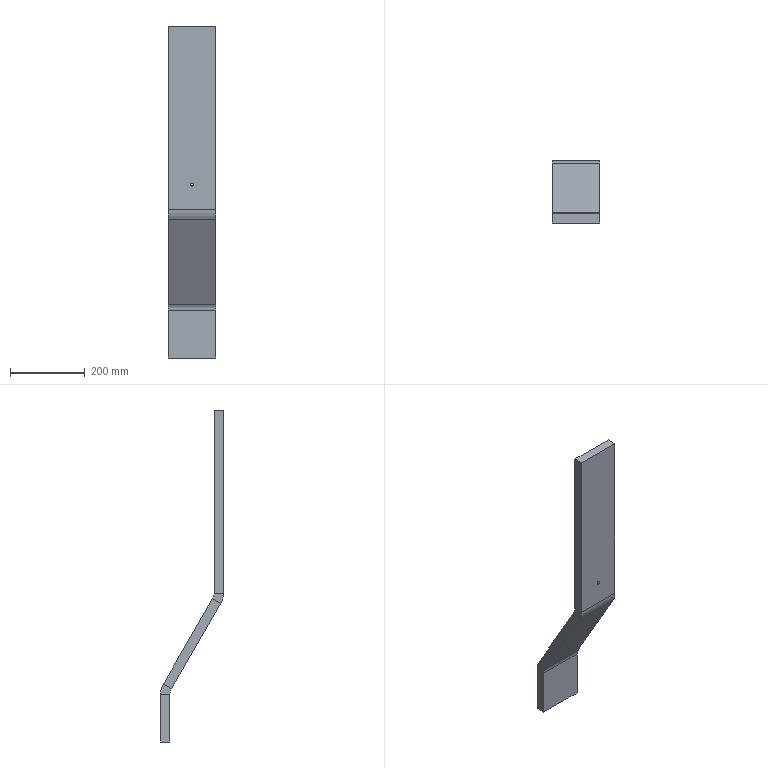Part | SolidWorks | features FlatPattern 1, ICE 1, SMBaseFlange 1, SheetMetal 1 | 1 solid | 24 faces | box 126 x 168 x 887 mm | volume 2910198 mm3 | plane 18 | cylinder 6 | commonest cylinder face diameters 8 x2 60 x2 110 x2
STEP:
#1=CARTESIAN_POINT('',(0.,-25.,-4.));
#2=VERTEX_POINT('',#1);
#3=CARTESIAN_POINT('',(0.,-25.,4.));
#4=VERTEX_POINT('',#3);
#5=CARTESIAN_POINT('',(0.,-25.,0.));
#6=DIRECTION('',(0.,1.,0.));
#7=DIRECTION('',(0.,0.,1.));
#8=AXIS2_PLACEMENT_3D('',#5,#6,#7);
#9=CIRCLE('',#8,4.);
#10=EDGE_CURVE('',#2,#4,#9,.T.);
#11=ORIENTED_EDGE('',*,*,#10,.F.);
#12=CARTESIAN_POINT('',(0.,0.,-4.));
#13=VERTEX_POINT('',#12);
#14=CARTESIAN_POINT('',(0.,-25.,-4.));
#15=DIRECTION('',(0.,1.,0.));
#16=VECTOR('',#15,1000.);
#17=LINE('',#14,#16);
#18=EDGE_CURVE('',#2,#13,#17,.T.);
#19=ORIENTED_EDGE('',*,*,#18,.T.);
#20=CARTESIAN_POINT('',(0.,0.,4.));
#21=VERTEX_POINT('',#20);
#22=CARTESIAN_POINT('',(0.,0.,0.));
#23=DIRECTION('',(0.,1.,0.));
#24=DIRECTION('',(0.,0.,1.));
#25=AXIS2_PLACEMENT_3D('',#22,#23,#24);
#26=CIRCLE('',#25,4.);
#27=EDGE_CURVE('',#13,#21,#26,.T.);
#28=ORIENTED_EDGE('',*,*,#27,.T.);
#29=CARTESIAN_POINT('',(0.,-25.,4.));
#30=DIRECTION('',(0.,1.,0.));
#31=VECTOR('',#30,1000.);
#32=LINE('',#29,#31);
#33=EDGE_CURVE('',#4,#21,#32,.T.);
#34=ORIENTED_EDGE('',*,*,#33,.F.);
#35=EDGE_LOOP('',(#11,#19,#28,#34));
#36=FACE_OUTER_BOUND('',#35,.T.);
#37=CARTESIAN_POINT('',(0.,-25.,0.));
#38=DIRECTION('',(0.,1.,0.));
#39=DIRECTION('',(0.,0.,1.));
#40=AXIS2_PLACEMENT_3D('',#37,#38,#39);
#41=CYLINDRICAL_SURFACE('',#40,4.);
#42=ADVANCED_FACE('',(#36),#41,.F.);
#43=CARTESIAN_POINT('',(63.,-25.,-65.263));
#44=VERTEX_POINT('',#43);
#45=CARTESIAN_POINT('',(63.,0.,-65.263));
#46=VERTEX_POINT('',#45);
#47=CARTESIAN_POINT('',(63.,-25.,-65.263));
#48=DIRECTION('',(0.,1.,0.));
#49=VECTOR('',#48,1000.);
#50=LINE('',#47,#49);
#51=EDGE_CURVE('',#44,#46,#50,.T.);
#52=ORIENTED_EDGE('',*,*,#51,.F.);
#53=CARTESIAN_POINT('',(63.,-17.631,-92.763));
#54=VERTEX_POINT('',#53);
#55=CARTESIAN_POINT('',(63.,30.,-65.263));
#56=DIRECTION('',(1.,0.,0.));
#57=DIRECTION('',(0.,0.,1.));
#58=AXIS2_PLACEMENT_3D('',#55,#56,#57);
#59=CIRCLE('',#58,55.);
#60=EDGE_CURVE('',#44,#54,#59,.T.);
#61=ORIENTED_EDGE('',*,*,#60,.T.);
#62=CARTESIAN_POINT('',(63.,4.019,-80.263));
#63=VERTEX_POINT('',#62);
#64=CARTESIAN_POINT('',(63.,4.019,-80.263));
#65=DIRECTION('',(0.,-0.866,-0.5));
#66=VECTOR('',#65,1000.);
#67=LINE('',#64,#66);
#68=EDGE_CURVE('',#63,#54,#67,.T.);
#69=ORIENTED_EDGE('',*,*,#68,.F.);
#70=CARTESIAN_POINT('',(63.,30.,-65.263));
#71=DIRECTION('',(1.,0.,0.));
#72=DIRECTION('',(0.,0.,-1.));
#73=AXIS2_PLACEMENT_3D('',#70,#71,#72);
#74=CIRCLE('',#73,30.);
#75=EDGE_CURVE('',#46,#63,#74,.T.);
#76=ORIENTED_EDGE('',*,*,#75,.F.);
#77=EDGE_LOOP('',(#52,#61,#69,#76));
#78=FACE_OUTER_BOUND('',#77,.T.);
#79=CARTESIAN_POINT('',(63.,-25.,-65.263));
#80=DIRECTION('',(1.,0.,0.));
#81=DIRECTION('',(0.,0.,-1.));
#82=AXIS2_PLACEMENT_3D('',#79,#80,#81);
#83=PLANE('',#82);
#84=ADVANCED_FACE('',(#78),#83,.T.);
#85=CARTESIAN_POINT('',(63.,-25.,424.));
#86=VERTEX_POINT('',#85);
#87=CARTESIAN_POINT('',(63.,-25.,424.));
#88=DIRECTION('',(0.,0.,-1.));
#89=VECTOR('',#88,1000.);
#90=LINE('',#87,#89);
#91=EDGE_CURVE('',#86,#44,#90,.T.);
#92=ORIENTED_EDGE('',*,*,#91,.T.);
#93=ORIENTED_EDGE('',*,*,#51,.T.);
#94=CARTESIAN_POINT('',(63.,0.,424.));
#95=VERTEX_POINT('',#94);
#96=CARTESIAN_POINT('',(63.,0.,424.));
#97=DIRECTION('',(0.,0.,-1.));
#98=VECTOR('',#97,1000.);
#99=LINE('',#96,#98);
#100=EDGE_CURVE('',#95,#46,#99,.T.);
#101=ORIENTED_EDGE('',*,*,#100,.F.);
#102=CARTESIAN_POINT('',(63.,-25.,424.));
#103=DIRECTION('',(0.,1.,0.));
#104=VECTOR('',#103,1000.);
#105=LINE('',#102,#104);
#106=EDGE_CURVE('',#86,#95,#105,.T.);
#107=ORIENTED_EDGE('',*,*,#106,.F.);
#108=EDGE_LOOP('',(#92,#93,#101,#107));
#109=FACE_OUTER_BOUND('',#108,.T.);
#110=CARTESIAN_POINT('',(63.,4.019,-80.263));
#111=DIRECTION('',(1.,0.,0.));
#112=DIRECTION('',(0.,0.,-1.));
#113=AXIS2_PLACEMENT_3D('',#110,#111,#112);
#114=PLANE('',#113);
#115=ADVANCED_FACE('',(#109),#114,.T.);
#116=CARTESIAN_POINT('',(-63.,-17.631,-92.763));
#117=VERTEX_POINT('',#116);
#118=CARTESIAN_POINT('',(-63.,4.019,-80.263));
#119=VERTEX_POINT('',#118);
#120=CARTESIAN_POINT('',(-63.,-17.631,-92.763));
#121=DIRECTION('',(0.,0.866,0.5));
#122=VECTOR('',#121,1000.);
#123=LINE('',#120,#122);
#124=EDGE_CURVE('',#117,#119,#123,.T.);
#125=ORIENTED_EDGE('',*,*,#124,.F.);
#126=CARTESIAN_POINT('',(-63.,-25.,-65.263));
#127=VERTEX_POINT('',#126);
#128=CARTESIAN_POINT('',(-63.,30.,-65.263));
#129=DIRECTION('',(1.,0.,0.));
#130=DIRECTION('',(0.,0.,1.));
#131=AXIS2_PLACEMENT_3D('',#128,#129,#130);
#132=CIRCLE('',#131,55.);
#133=EDGE_CURVE('',#127,#117,#132,.T.);
#134=ORIENTED_EDGE('',*,*,#133,.F.);
#135=CARTESIAN_POINT('',(-63.,0.,-65.263));
#136=VERTEX_POINT('',#135);
#137=CARTESIAN_POINT('',(-63.,0.,-65.263));
#138=DIRECTION('',(0.,-1.,0.));
#139=VECTOR('',#138,1000.);
#140=LINE('',#137,#139);
#141=EDGE_CURVE('',#136,#127,#140,.T.);
#142=ORIENTED_EDGE('',*,*,#141,.F.);
#143=CARTESIAN_POINT('',(-63.,30.,-65.263));
#144=DIRECTION('',(1.,0.,0.));
#145=DIRECTION('',(0.,0.,-1.));
#146=AXIS2_PLACEMENT_3D('',#143,#144,#145);
#147=CIRCLE('',#146,30.);
#148=EDGE_CURVE('',#136,#119,#147,.T.);
#149=ORIENTED_EDGE('',*,*,#148,.T.);
#150=EDGE_LOOP('',(#125,#134,#142,#149));
#151=FACE_OUTER_BOUND('',#150,.T.);
#152=CARTESIAN_POINT('',(-63.,-17.631,-92.763));
#153=DIRECTION('',(-1.,0.,0.));
#154=DIRECTION('',(0.,0.,1.));
#155=AXIS2_PLACEMENT_3D('',#152,#153,#154);
#156=PLANE('',#155);
#157=ADVANCED_FACE('',(#151),#156,.T.);
#158=CARTESIAN_POINT('',(-63.,113.981,-320.722));
#159=VERTEX_POINT('',#158);
#160=CARTESIAN_POINT('',(-63.,-25.,-80.));
#161=DIRECTION('',(0.,0.5,-0.866));
#162=VECTOR('',#161,1000.);
#163=LINE('',#160,#162);
#164=EDGE_CURVE('',#117,#159,#163,.T.);
#165=ORIENTED_EDGE('',*,*,#164,.F.);
#166=ORIENTED_EDGE('',*,*,#124,.T.);
#167=CARTESIAN_POINT('',(-63.,135.631,-308.222));
#168=VERTEX_POINT('',#167);
#169=CARTESIAN_POINT('',(-63.,-3.349,-67.5));
#170=DIRECTION('',(0.,0.5,-0.866));
#171=VECTOR('',#170,1000.);
#172=LINE('',#169,#171);
#173=EDGE_CURVE('',#119,#168,#172,.T.);
#174=ORIENTED_EDGE('',*,*,#173,.T.);
#175=CARTESIAN_POINT('',(-63.,135.631,-308.222));
#176=DIRECTION('',(0.,-0.866,-0.5));
#177=VECTOR('',#176,1000.);
#178=LINE('',#175,#177);
#179=EDGE_CURVE('',#168,#159,#178,.T.);
#180=ORIENTED_EDGE('',*,*,#179,.T.);
#181=EDGE_LOOP('',(#165,#166,#174,#180));
#182=FACE_OUTER_BOUND('',#181,.T.);
#183=CARTESIAN_POINT('',(-63.,0.,-65.263));
#184=DIRECTION('',(-1.,0.,0.));
#185=DIRECTION('',(0.,0.,1.));
#186=AXIS2_PLACEMENT_3D('',#183,#184,#185);
#187=PLANE('',#186);
#188=ADVANCED_FACE('',(#182),#187,.T.);
#189=CARTESIAN_POINT('',(63.,113.981,-320.722));
#190=VERTEX_POINT('',#189);
#191=CARTESIAN_POINT('',(63.,135.631,-308.222));
#192=VERTEX_POINT('',#191);
#193=CARTESIAN_POINT('',(63.,113.981,-320.722));
#194=DIRECTION('',(0.,0.866,0.5));
#195=VECTOR('',#194,1000.);
#196=LINE('',#193,#195);
#197=EDGE_CURVE('',#190,#192,#196,.T.);
#198=ORIENTED_EDGE('',*,*,#197,.F.);
#199=CARTESIAN_POINT('',(63.,118.,-335.722));
#200=VERTEX_POINT('',#199);
#201=CARTESIAN_POINT('',(63.,88.,-335.722));
#202=DIRECTION('',(-1.,0.,0.));
#203=DIRECTION('',(0.,0.,-1.));
#204=AXIS2_PLACEMENT_3D('',#201,#202,#203);
#205=CIRCLE('',#204,30.);
#206=EDGE_CURVE('',#190,#200,#205,.T.);
#207=ORIENTED_EDGE('',*,*,#206,.T.);
#208=CARTESIAN_POINT('',(63.,143.,-335.722));
#209=VERTEX_POINT('',#208);
#210=CARTESIAN_POINT('',(63.,143.,-335.722));
#211=DIRECTION('',(0.,-1.,0.));
#212=VECTOR('',#211,1000.);
#213=LINE('',#210,#212);
#214=EDGE_CURVE('',#209,#200,#213,.T.);
#215=ORIENTED_EDGE('',*,*,#214,.F.);
#216=CARTESIAN_POINT('',(63.,88.,-335.722));
#217=DIRECTION('',(-1.,0.,0.));
#218=DIRECTION('',(0.,0.,-1.));
#219=AXIS2_PLACEMENT_3D('',#216,#217,#218);
#220=CIRCLE('',#219,55.);
#221=EDGE_CURVE('',#192,#209,#220,.T.);
#222=ORIENTED_EDGE('',*,*,#221,.F.);
#223=EDGE_LOOP('',(#198,#207,#215,#222));
#224=FACE_OUTER_BOUND('',#223,.T.);
#225=CARTESIAN_POINT('',(63.,113.981,-320.722));
#226=DIRECTION('',(1.,0.,0.));
#227=DIRECTION('',(0.,0.,-1.));
#228=AXIS2_PLACEMENT_3D('',#225,#226,#227);
#229=PLANE('',#228);
#230=ADVANCED_FACE('',(#224),#229,.T.);
#231=CARTESIAN_POINT('',(63.,-25.,-80.));
#232=DIRECTION('',(0.,0.5,-0.866));
#233=VECTOR('',#232,1000.);
#234=LINE('',#231,#233);
#235=EDGE_CURVE('',#54,#190,#234,.T.);
#236=ORIENTED_EDGE('',*,*,#235,.T.);
#237=ORIENTED_EDGE('',*,*,#197,.T.);
#238=CARTESIAN_POINT('',(63.,-3.349,-67.5));
#239=DIRECTION('',(0.,0.5,-0.866));
#240=VECTOR('',#239,1000.);
#241=LINE('',#238,#240);
#242=EDGE_CURVE('',#63,#192,#241,.T.);
#243=ORIENTED_EDGE('',*,*,#242,.F.);
#244=ORIENTED_EDGE('',*,*,#68,.T.);
#245=EDGE_LOOP('',(#236,#237,#243,#244));
#246=FACE_OUTER_BOUND('',#245,.T.);
#247=CARTESIAN_POINT('',(63.,143.,-335.722));
#248=DIRECTION('',(1.,0.,0.));
#249=DIRECTION('',(0.,0.,-1.));
#250=AXIS2_PLACEMENT_3D('',#247,#248,#249);
#251=PLANE('',#250);
#252=ADVANCED_FACE('',(#246),#251,.T.);
#253=CARTESIAN_POINT('',(-63.,118.,-335.722));
#254=VERTEX_POINT('',#253);
#255=CARTESIAN_POINT('',(-63.,143.,-335.722));
#256=VERTEX_POINT('',#255);
#257=CARTESIAN_POINT('',(-63.,118.,-335.722));
#258=DIRECTION('',(0.,1.,0.));
#259=VECTOR('',#258,1000.);
#260=LINE('',#257,#259);
#261=EDGE_CURVE('',#254,#256,#260,.T.);
#262=ORIENTED_EDGE('',*,*,#261,.F.);
#263=CARTESIAN_POINT('',(-63.,88.,-335.722));
#264=DIRECTION('',(-1.,0.,0.));
#265=DIRECTION('',(0.,0.,-1.));
#266=AXIS2_PLACEMENT_3D('',#263,#264,#265);
#267=CIRCLE('',#266,30.);
#268=EDGE_CURVE('',#159,#254,#267,.T.);
#269=ORIENTED_EDGE('',*,*,#268,.F.);
#270=ORIENTED_EDGE('',*,*,#179,.F.);
#271=CARTESIAN_POINT('',(-63.,88.,-335.722));
#272=DIRECTION('',(-1.,0.,0.));
#273=DIRECTION('',(0.,0.,-1.));
#274=AXIS2_PLACEMENT_3D('',#271,#272,#273);
#275=CIRCLE('',#274,55.);
#276=EDGE_CURVE('',#168,#256,#275,.T.);
#277=ORIENTED_EDGE('',*,*,#276,.T.);
#278=EDGE_LOOP('',(#262,#269,#270,#277));
#279=FACE_OUTER_BOUND('',#278,.T.);
#280=CARTESIAN_POINT('',(-63.,118.,-335.722));
#281=DIRECTION('',(-1.,0.,0.));
#282=DIRECTION('',(0.,0.,1.));
#283=AXIS2_PLACEMENT_3D('',#280,#281,#282);
#284=PLANE('',#283);
#285=ADVANCED_FACE('',(#279),#284,.T.);
#286=CARTESIAN_POINT('',(-63.,118.,-463.));
#287=VERTEX_POINT('',#286);
#288=CARTESIAN_POINT('',(-63.,118.,-327.683));
#289=DIRECTION('',(0.,0.,-1.));
#290=VECTOR('',#289,1000.);
#291=LINE('',#288,#290);
#292=EDGE_CURVE('',#254,#287,#291,.T.);
#293=ORIENTED_EDGE('',*,*,#292,.F.);
#294=ORIENTED_EDGE('',*,*,#261,.T.);
#295=CARTESIAN_POINT('',(-63.,143.,-463.));
#296=VERTEX_POINT('',#295);
#297=CARTESIAN_POINT('',(-63.,143.,-327.683));
#298=DIRECTION('',(0.,0.,-1.));
#299=VECTOR('',#298,1000.);
#300=LINE('',#297,#299);
#301=EDGE_CURVE('',#256,#296,#300,.T.);
#302=ORIENTED_EDGE('',*,*,#301,.T.);
#303=CARTESIAN_POINT('',(-63.,143.,-463.));
#304=DIRECTION('',(0.,-1.,0.));
#305=VECTOR('',#304,1000.);
#306=LINE('',#303,#305);
#307=EDGE_CURVE('',#296,#287,#306,.T.);
#308=ORIENTED_EDGE('',*,*,#307,.T.);
#309=EDGE_LOOP('',(#293,#294,#302,#308));
#310=FACE_OUTER_BOUND('',#309,.T.);
#311=CARTESIAN_POINT('',(-63.,135.631,-308.222));
#312=DIRECTION('',(-1.,0.,0.));
#313=DIRECTION('',(0.,0.,1.));
#314=AXIS2_PLACEMENT_3D('',#311,#312,#313);
#315=PLANE('',#314);
#316=ADVANCED_FACE('',(#310),#315,.T.);
#317=ORIENTED_EDGE('',*,*,#292,.T.);
#318=CARTESIAN_POINT('',(63.,118.,-463.));
#319=VERTEX_POINT('',#318);
#320=CARTESIAN_POINT('',(63.,118.,-463.));
#321=DIRECTION('',(-1.,0.,0.));
#322=VECTOR('',#321,1000.);
#323=LINE('',#320,#322);
#324=EDGE_CURVE('',#319,#287,#323,.T.);
#325=ORIENTED_EDGE('',*,*,#324,.F.);
#326=CARTESIAN_POINT('',(63.,118.,-327.683));
#327=DIRECTION('',(0.,0.,-1.));
#328=VECTOR('',#327,1000.);
#329=LINE('',#326,#328);
#330=EDGE_CURVE('',#200,#319,#329,.T.);
#331=ORIENTED_EDGE('',*,*,#330,.F.);
#332=CARTESIAN_POINT('',(63.,118.,-335.722));
#333=DIRECTION('',(-1.,0.,0.));
#334=VECTOR('',#333,1000.);
#335=LINE('',#332,#334);
#336=EDGE_CURVE('',#200,#254,#335,.T.);
#337=ORIENTED_EDGE('',*,*,#336,.T.);
#338=EDGE_LOOP('',(#317,#325,#331,#337));
#339=FACE_OUTER_BOUND('',#338,.T.);
#340=CARTESIAN_POINT('',(63.,118.,-327.683));
#341=DIRECTION('',(0.,1.,0.));
#342=DIRECTION('',(0.,0.,1.));
#343=AXIS2_PLACEMENT_3D('',#340,#341,#342);
#344=PLANE('',#343);
#345=ADVANCED_FACE('',(#339),#344,.F.);
#346=ORIENTED_EDGE('',*,*,#307,.F.);
#347=CARTESIAN_POINT('',(63.,143.,-463.));
#348=VERTEX_POINT('',#347);
#349=CARTESIAN_POINT('',(63.,143.,-463.));
#350=DIRECTION('',(-1.,0.,0.));
#351=VECTOR('',#350,1000.);
#352=LINE('',#349,#351);
#353=EDGE_CURVE('',#348,#296,#352,.T.);
#354=ORIENTED_EDGE('',*,*,#353,.F.);
#355=CARTESIAN_POINT('',(63.,143.,-463.));
#356=DIRECTION('',(0.,-1.,0.));
#357=VECTOR('',#356,1000.);
#358=LINE('',#355,#357);
#359=EDGE_CURVE('',#348,#319,#358,.T.);
#360=ORIENTED_EDGE('',*,*,#359,.T.);
#361=ORIENTED_EDGE('',*,*,#324,.T.);
#362=EDGE_LOOP('',(#346,#354,#360,#361));
#363=FACE_OUTER_BOUND('',#362,.T.);
#364=CARTESIAN_POINT('',(63.,143.,-463.));
#365=DIRECTION('',(0.,0.,-1.));
#366=DIRECTION('',(-1.,0.,0.));
#367=AXIS2_PLACEMENT_3D('',#364,#365,#366);
#368=PLANE('',#367);
#369=ADVANCED_FACE('',(#363),#368,.T.);
#370=ORIENTED_EDGE('',*,*,#301,.F.);
#371=CARTESIAN_POINT('',(63.,143.,-335.722));
#372=DIRECTION('',(-1.,0.,0.));
#373=VECTOR('',#372,1000.);
#374=LINE('',#371,#373);
#375=EDGE_CURVE('',#209,#256,#374,.T.);
#376=ORIENTED_EDGE('',*,*,#375,.F.);
#377=CARTESIAN_POINT('',(63.,143.,-327.683));
#378=DIRECTION('',(0.,0.,-1.));
#379=VECTOR('',#378,1000.);
#380=LINE('',#377,#379);
#381=EDGE_CURVE('',#209,#348,#380,.T.);
#382=ORIENTED_EDGE('',*,*,#381,.T.);
#383=ORIENTED_EDGE('',*,*,#353,.T.);
#384=EDGE_LOOP('',(#370,#376,#382,#383));
#385=FACE_OUTER_BOUND('',#384,.T.);
#386=CARTESIAN_POINT('',(63.,143.,-327.683));
#387=DIRECTION('',(0.,1.,0.));
#388=DIRECTION('',(0.,0.,1.));
#389=AXIS2_PLACEMENT_3D('',#386,#387,#388);
#390=PLANE('',#389);
#391=ADVANCED_FACE('',(#385),#390,.T.);
#392=ORIENTED_EDGE('',*,*,#276,.F.);
#393=CARTESIAN_POINT('',(63.,135.631,-308.222));
#394=DIRECTION('',(-1.,0.,0.));
#395=VECTOR('',#394,1000.);
#396=LINE('',#393,#395);
#397=EDGE_CURVE('',#192,#168,#396,.T.);
#398=ORIENTED_EDGE('',*,*,#397,.F.);
#399=ORIENTED_EDGE('',*,*,#221,.T.);
#400=ORIENTED_EDGE('',*,*,#375,.T.);
#401=EDGE_LOOP('',(#392,#398,#399,#400));
#402=FACE_OUTER_BOUND('',#401,.T.);
#403=CARTESIAN_POINT('',(63.,88.,-335.722));
#404=DIRECTION('',(-1.,0.,0.));
#405=DIRECTION('',(0.,0.,1.));
#406=AXIS2_PLACEMENT_3D('',#403,#404,#405);
#407=CYLINDRICAL_SURFACE('',#406,55.);
#408=ADVANCED_FACE('',(#402),#407,.T.);
#409=ORIENTED_EDGE('',*,*,#173,.F.);
#410=CARTESIAN_POINT('',(63.,4.019,-80.263));
#411=DIRECTION('',(-1.,0.,0.));
#412=VECTOR('',#411,1000.);
#413=LINE('',#410,#412);
#414=EDGE_CURVE('',#63,#119,#413,.T.);
#415=ORIENTED_EDGE('',*,*,#414,.F.);
#416=ORIENTED_EDGE('',*,*,#242,.T.);
#417=ORIENTED_EDGE('',*,*,#397,.T.);
#418=EDGE_LOOP('',(#409,#415,#416,#417));
#419=FACE_OUTER_BOUND('',#418,.T.);
#420=CARTESIAN_POINT('',(63.,-3.349,-67.5));
#421=DIRECTION('',(0.,0.866,0.5));
#422=DIRECTION('',(0.,-0.5,0.866));
#423=AXIS2_PLACEMENT_3D('',#420,#421,#422);
#424=PLANE('',#423);
#425=ADVANCED_FACE('',(#419),#424,.T.);
#426=ORIENTED_EDGE('',*,*,#148,.F.);
#427=CARTESIAN_POINT('',(63.,0.,-65.263));
#428=DIRECTION('',(-1.,0.,0.));
#429=VECTOR('',#428,1000.);
#430=LINE('',#427,#429);
#431=EDGE_CURVE('',#46,#136,#430,.T.);
#432=ORIENTED_EDGE('',*,*,#431,.F.);
#433=ORIENTED_EDGE('',*,*,#75,.T.);
#434=ORIENTED_EDGE('',*,*,#414,.T.);
#435=EDGE_LOOP('',(#426,#432,#433,#434));
#436=FACE_OUTER_BOUND('',#435,.T.);
#437=CARTESIAN_POINT('',(63.,30.,-65.263));
#438=DIRECTION('',(-1.,0.,0.));
#439=DIRECTION('',(0.,0.,1.));
#440=AXIS2_PLACEMENT_3D('',#437,#438,#439);
#441=CYLINDRICAL_SURFACE('',#440,30.);
#442=ADVANCED_FACE('',(#436),#441,.F.);
#443=CARTESIAN_POINT('',(0.,0.,0.));
#444=DIRECTION('',(0.,1.,0.));
#445=DIRECTION('',(0.,0.,1.));
#446=AXIS2_PLACEMENT_3D('',#443,#444,#445);
#447=CIRCLE('',#446,4.);
#448=EDGE_CURVE('',#21,#13,#447,.T.);
#449=ORIENTED_EDGE('',*,*,#448,.F.);
#450=ORIENTED_EDGE('',*,*,#27,.F.);
#451=EDGE_LOOP('',(#449,#450));
#452=FACE_BOUND('',#451,.T.);
#453=CARTESIAN_POINT('',(-63.,0.,424.));
#454=VERTEX_POINT('',#453);
#455=CARTESIAN_POINT('',(-63.,0.,424.));
#456=DIRECTION('',(0.,0.,-1.));
#457=VECTOR('',#456,1000.);
#458=LINE('',#455,#457);
#459=EDGE_CURVE('',#454,#136,#458,.T.);
#460=ORIENTED_EDGE('',*,*,#459,.F.);
#461=CARTESIAN_POINT('',(63.,0.,424.));
#462=DIRECTION('',(-1.,0.,0.));
#463=VECTOR('',#462,1000.);
#464=LINE('',#461,#463);
#465=EDGE_CURVE('',#95,#454,#464,.T.);
#466=ORIENTED_EDGE('',*,*,#465,.F.);
#467=ORIENTED_EDGE('',*,*,#100,.T.);
#468=ORIENTED_EDGE('',*,*,#431,.T.);
#469=EDGE_LOOP('',(#460,#466,#467,#468));
#470=FACE_OUTER_BOUND('',#469,.T.);
#471=CARTESIAN_POINT('',(63.,0.,424.));
#472=DIRECTION('',(0.,1.,0.));
#473=DIRECTION('',(0.,0.,1.));
#474=AXIS2_PLACEMENT_3D('',#471,#472,#473);
#475=PLANE('',#474);
#476=ADVANCED_FACE('',(#452,#470),#475,.T.);
#477=CARTESIAN_POINT('',(-63.,-25.,424.));
#478=VERTEX_POINT('',#477);
#479=CARTESIAN_POINT('',(-63.,-25.,424.));
#480=DIRECTION('',(0.,1.,0.));
#481=VECTOR('',#480,1000.);
#482=LINE('',#479,#481);
#483=EDGE_CURVE('',#478,#454,#482,.T.);
#484=ORIENTED_EDGE('',*,*,#483,.F.);
#485=CARTESIAN_POINT('',(63.,-25.,424.));
#486=DIRECTION('',(-1.,0.,0.));
#487=VECTOR('',#486,1000.);
#488=LINE('',#485,#487);
#489=EDGE_CURVE('',#86,#478,#488,.T.);
#490=ORIENTED_EDGE('',*,*,#489,.F.);
#491=ORIENTED_EDGE('',*,*,#106,.T.);
#492=ORIENTED_EDGE('',*,*,#465,.T.);
#493=EDGE_LOOP('',(#484,#490,#491,#492));
#494=FACE_OUTER_BOUND('',#493,.T.);
#495=CARTESIAN_POINT('',(63.,-25.,424.));
#496=DIRECTION('',(0.,0.,1.));
#497=DIRECTION('',(1.,0.,0.));
#498=AXIS2_PLACEMENT_3D('',#495,#496,#497);
#499=PLANE('',#498);
#500=ADVANCED_FACE('',(#494),#499,.T.);
#501=CARTESIAN_POINT('',(0.,-25.,0.));
#502=DIRECTION('',(0.,1.,0.));
#503=DIRECTION('',(0.,0.,1.));
#504=AXIS2_PLACEMENT_3D('',#501,#502,#503);
#505=CIRCLE('',#504,4.);
#506=EDGE_CURVE('',#4,#2,#505,.T.);
#507=ORIENTED_EDGE('',*,*,#506,.T.);
#508=ORIENTED_EDGE('',*,*,#10,.T.);
#509=EDGE_LOOP('',(#507,#508));
#510=FACE_BOUND('',#509,.T.);
#511=CARTESIAN_POINT('',(-63.,-25.,424.));
#512=DIRECTION('',(0.,0.,-1.));
#513=VECTOR('',#512,1000.);
#514=LINE('',#511,#513);
#515=EDGE_CURVE('',#478,#127,#514,.T.);
#516=ORIENTED_EDGE('',*,*,#515,.T.);
#517=CARTESIAN_POINT('',(63.,-25.,-65.263));
#518=DIRECTION('',(-1.,0.,0.));
#519=VECTOR('',#518,1000.);
#520=LINE('',#517,#519);
#521=EDGE_CURVE('',#44,#127,#520,.T.);
#522=ORIENTED_EDGE('',*,*,#521,.F.);
#523=ORIENTED_EDGE('',*,*,#91,.F.);
#524=ORIENTED_EDGE('',*,*,#489,.T.);
#525=EDGE_LOOP('',(#516,#522,#523,#524));
#526=FACE_OUTER_BOUND('',#525,.T.);
#527=CARTESIAN_POINT('',(63.,-25.,424.));
#528=DIRECTION('',(0.,1.,0.));
#529=DIRECTION('',(0.,0.,1.));
#530=AXIS2_PLACEMENT_3D('',#527,#528,#529);
#531=PLANE('',#530);
#532=ADVANCED_FACE('',(#510,#526),#531,.F.);
#533=ORIENTED_EDGE('',*,*,#133,.T.);
#534=CARTESIAN_POINT('',(63.,-17.631,-92.763));
#535=DIRECTION('',(-1.,0.,0.));
#536=VECTOR('',#535,1000.);
#537=LINE('',#534,#536);
#538=EDGE_CURVE('',#54,#117,#537,.T.);
#539=ORIENTED_EDGE('',*,*,#538,.F.);
#540=ORIENTED_EDGE('',*,*,#60,.F.);
#541=ORIENTED_EDGE('',*,*,#521,.T.);
#542=EDGE_LOOP('',(#533,#539,#540,#541));
#543=FACE_OUTER_BOUND('',#542,.T.);
#544=CARTESIAN_POINT('',(63.,30.,-65.263));
#545=DIRECTION('',(-1.,0.,0.));
#546=DIRECTION('',(0.,0.,1.));
#547=AXIS2_PLACEMENT_3D('',#544,#545,#546);
#548=CYLINDRICAL_SURFACE('',#547,55.);
#549=ADVANCED_FACE('',(#543),#548,.T.);
#550=ORIENTED_EDGE('',*,*,#164,.T.);
#551=CARTESIAN_POINT('',(63.,113.981,-320.722));
#552=DIRECTION('',(-1.,0.,0.));
#553=VECTOR('',#552,1000.);
#554=LINE('',#551,#553);
#555=EDGE_CURVE('',#190,#159,#554,.T.);
#556=ORIENTED_EDGE('',*,*,#555,.F.);
#557=ORIENTED_EDGE('',*,*,#235,.F.);
#558=ORIENTED_EDGE('',*,*,#538,.T.);
#559=EDGE_LOOP('',(#550,#556,#557,#558));
#560=FACE_OUTER_BOUND('',#559,.T.);
#561=CARTESIAN_POINT('',(63.,-25.,-80.));
#562=DIRECTION('',(0.,0.866,0.5));
#563=DIRECTION('',(0.,-0.5,0.866));
#564=AXIS2_PLACEMENT_3D('',#561,#562,#563);
#565=PLANE('',#564);
#566=ADVANCED_FACE('',(#560),#565,.F.);
#567=ORIENTED_EDGE('',*,*,#268,.T.);
#568=ORIENTED_EDGE('',*,*,#336,.F.);
#569=ORIENTED_EDGE('',*,*,#206,.F.);
#570=ORIENTED_EDGE('',*,*,#555,.T.);
#571=EDGE_LOOP('',(#567,#568,#569,#570));
#572=FACE_OUTER_BOUND('',#571,.T.);
#573=CARTESIAN_POINT('',(63.,88.,-335.722));
#574=DIRECTION('',(-1.,0.,0.));
#575=DIRECTION('',(0.,0.,1.));
#576=AXIS2_PLACEMENT_3D('',#573,#574,#575);
#577=CYLINDRICAL_SURFACE('',#576,30.);
#578=ADVANCED_FACE('',(#572),#577,.F.);
#579=ORIENTED_EDGE('',*,*,#330,.T.);
#580=ORIENTED_EDGE('',*,*,#359,.F.);
#581=ORIENTED_EDGE('',*,*,#381,.F.);
#582=ORIENTED_EDGE('',*,*,#214,.T.);
#583=EDGE_LOOP('',(#579,#580,#581,#582));
#584=FACE_OUTER_BOUND('',#583,.T.);
#585=CARTESIAN_POINT('',(63.,88.,-335.722));
#586=DIRECTION('',(1.,0.,0.));
#587=DIRECTION('',(0.,0.,-1.));
#588=AXIS2_PLACEMENT_3D('',#585,#586,#587);
#589=PLANE('',#588);
#590=ADVANCED_FACE('',(#584),#589,.T.);
#591=ORIENTED_EDGE('',*,*,#459,.T.);
#592=ORIENTED_EDGE('',*,*,#141,.T.);
#593=ORIENTED_EDGE('',*,*,#515,.F.);
#594=ORIENTED_EDGE('',*,*,#483,.T.);
#595=EDGE_LOOP('',(#591,#592,#593,#594));
#596=FACE_OUTER_BOUND('',#595,.T.);
#597=CARTESIAN_POINT('',(-63.,88.,-335.722));
#598=DIRECTION('',(1.,0.,0.));
#599=DIRECTION('',(0.,0.,-1.));
#600=AXIS2_PLACEMENT_3D('',#597,#598,#599);
#601=PLANE('',#600);
#602=ADVANCED_FACE('',(#596),#601,.F.);
#603=ORIENTED_EDGE('',*,*,#18,.F.);
#604=ORIENTED_EDGE('',*,*,#506,.F.);
#605=ORIENTED_EDGE('',*,*,#33,.T.);
#606=ORIENTED_EDGE('',*,*,#448,.T.);
#607=EDGE_LOOP('',(#603,#604,#605,#606));
#608=FACE_OUTER_BOUND('',#607,.T.);
#609=CARTESIAN_POINT('',(0.,-25.,0.));
#610=DIRECTION('',(0.,1.,0.));
#611=DIRECTION('',(0.,0.,1.));
#612=AXIS2_PLACEMENT_3D('',#609,#610,#611);
#613=CYLINDRICAL_SURFACE('',#612,4.);
#614=ADVANCED_FACE('',(#608),#613,.F.);
#615=CLOSED_SHELL('',(#42,#84,#115,#157,#188,#230,#252,#285,#316,#345,#369,#391,#408,#425,#442,#476,#500,#532,#549,#566,#578,#590,#602,#614));
#616=MANIFOLD_SOLID_BREP('',#615);
#617=CARTESIAN_POINT('',(0.,0.,0.));
#618=DIRECTION('',(0.,0.,1.));
#619=DIRECTION('',(1.,0.,0.));
#620=AXIS2_PLACEMENT_3D('',#617,#618,#619);
#621=(LENGTH_UNIT()NAMED_UNIT(*)SI_UNIT(.MILLI.,.METRE.));
#622=UNCERTAINTY_MEASURE_WITH_UNIT(LENGTH_MEASURE(0.00001),#621,'','');
#623=(NAMED_UNIT(*)PLANE_ANGLE_UNIT()SI_UNIT($,.RADIAN.));
#624=(NAMED_UNIT(*)SI_UNIT($,.STERADIAN.)SOLID_ANGLE_UNIT());
#625=(GEOMETRIC_REPRESENTATION_CONTEXT(3)GLOBAL_UNCERTAINTY_ASSIGNED_CONTEXT((#622))GLOBAL_UNIT_ASSIGNED_CONTEXT((#621,#623,#624))REPRESENTATION_CONTEXT('',''));
#626=ADVANCED_BREP_SHAPE_REPRESENTATION('',(#616,#620),#625);